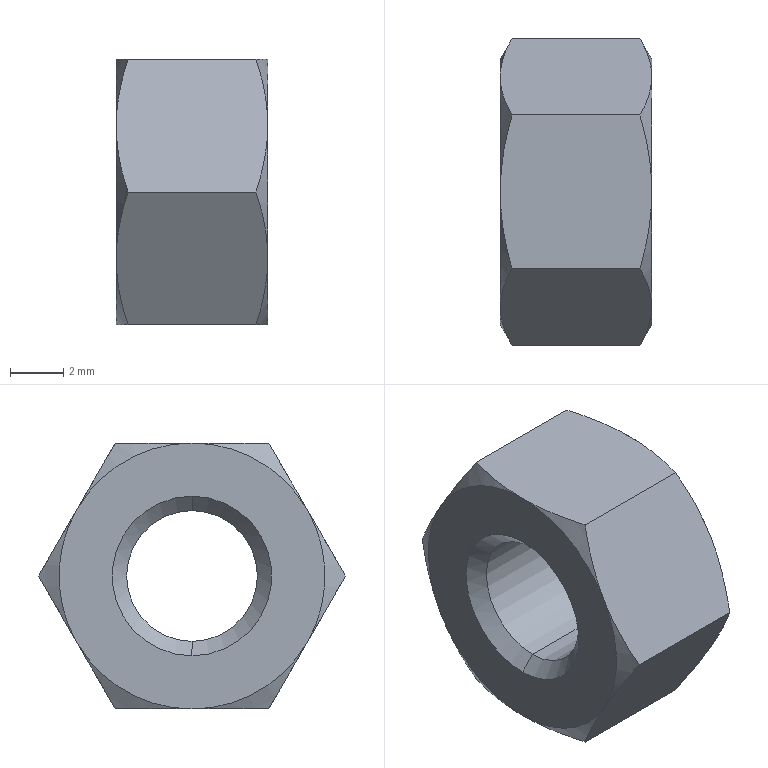Part | STEP file | 001-010-TBK32-M6 | 1 solid | 26 faces | box 5.7 x 11.547 x 10 mm | volume 378.382 mm3 | cone 16 | plane 8 | cylinder 2 | commonest cylinder face diameters 4.917 x2